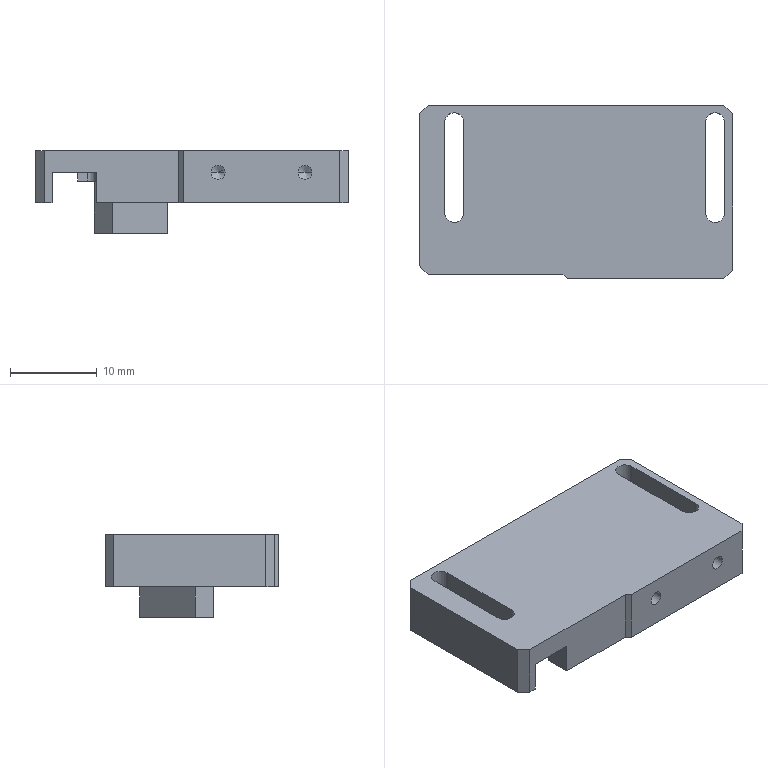NC program | NX | posted with a generic post | part box 36 x 20 x 9.5 mm
Lines 1 to 1629 of 4561:
N10 G17 G21 G94 G90
(FLOOR_WALL , TOOL : D10JING)
N12 T09 M6
N14 G54
N16 G17 G0 G90 X28. Y-11.997 S9500 M3
N18 G43 Z30. H9
N20 Z3.
N22 G94 G1 Z0. F1250.
N24 X25.
N26 X-25.
N28 Y-6.998
N30 X25.
N32 Y-1.999
N34 X-25.
N36 Y3.001
N38 X25.
N40 Y8.
N42 X-25.
N44 X-28.
N46 Z3.
N48 G0 Z30.
N50 M5
(ZLEVEL_PROFILE , TOOL : D10)
N52 T10 M6
N54 G54
N56 G17 G0 G90 X15.885 Y15.1 S9500 M3
N58 G43 Z30. H10
N60 Z1.5
N62 G94 G1 X17.554 Z1.413 F1000.
N64 X18.963 Y14.74 Z1.336
N66 X20.215 Y13.998 Z1.26
N68 X21.998 Y12.215 Z1.128
N70 X22.74 Y10.963 Z1.052
N72 X23.1 Y9.554 Z0.975
N74 Y-9.554 Z-0.026
N76 X22.74 Y-10.963 Z-0.102
N78 X21.998 Y-12.215 Z-0.178
N80 X20.215 Y-13.998 Z-0.311
N82 X18.963 Y-14.74 Z-0.387
N84 X17.554 Y-15.1 Z-0.463
N86 X17. Z-0.492
N88 X-17. F2500.
N90 G2 X-20.606 Y-13.606 R5.1
N92 G1 X-21.606 Y-12.606
N94 G2 X-23.1 Y-9. R5.1
N96 G1 Y8.5
N98 G2 X-21.606 Y12.106 R5.1
N100 G1 X-20.606 Y13.106
N102 G2 X-17. Y14.6 R5.1
N104 G1 X-3.202
N106 G2 X-1. Y15.1 R5.1
N108 G1 X17.
N110 G2 X20.606 Y13.606 R5.1
N112 G1 X21.606 Y12.606
N114 G2 X23.1 Y9. R5.1
N116 G1 Y-9.
N118 G2 X21.606 Y-12.606 R5.1
N120 G1 X20.606 Y-13.606
N122 G2 X17. Y-15.1 R5.1
N124 G1 X-11.193 Z-0.984
N126 X-17.
N128 G2 X-20.606 Y-13.606 R5.1
N130 G1 X-21.606 Y-12.606
N132 G2 X-23.1 Y-9. R5.1
N134 G1 Y8.5
N136 G2 X-21.606 Y12.106 R5.1
N138 G1 X-20.606 Y13.106
N140 G2 X-17. Y14.6 R5.1
N142 G1 X-3.202
N144 G2 X-1. Y15.1 R5.1
N146 G1 X17.
N148 G2 X20.606 Y13.606 R5.1
N150 G1 X21.606 Y12.606
N152 G2 X23.1 Y9. R5.1
N154 G1 Y-9.
N156 G2 X21.606 Y-12.606 R5.1
N158 G1 X20.606 Y-13.606
N160 G2 X17. Y-15.1 R5.1
N162 G1 X-11.193 Z-1.476
N164 X-17.
N166 G2 X-20.606 Y-13.606 R5.1
N168 G1 X-21.606 Y-12.606
N170 G2 X-23.1 Y-9. R5.1
N172 G1 Y8.5
N174 G2 X-21.606 Y12.106 R5.1
N176 G1 X-20.606 Y13.106
N178 G2 X-17. Y14.6 R5.1
N180 G1 X-3.202
N182 G2 X-1. Y15.1 R5.1
N184 G1 X17.
N186 G2 X20.606 Y13.606 R5.1
N188 G1 X21.606 Y12.606
N190 G2 X23.1 Y9. R5.1
N192 G1 Y-9.
N194 G2 X21.606 Y-12.606 R5.1
N196 G1 X20.606 Y-13.606
N198 G2 X17. Y-15.1 R5.1
N200 G1 X-11.193 Z-1.968
N202 X-17.
N204 G2 X-20.606 Y-13.606 R5.1
N206 G1 X-21.606 Y-12.606
N208 G2 X-23.1 Y-9. R5.1
N210 G1 Y8.5
N212 G2 X-21.606 Y12.106 R5.1
N214 G1 X-20.606 Y13.106
N216 G2 X-17. Y14.6 R5.1
N218 G1 X-3.202
N220 G2 X-1. Y15.1 R5.1
N222 G1 X17.
N224 G2 X20.606 Y13.606 R5.1
N226 G1 X21.606 Y12.606
N228 G2 X23.1 Y9. R5.1
N230 G1 Y-9.
N232 G2 X21.606 Y-12.606 R5.1
N234 G1 X20.606 Y-13.606
N236 G2 X17. Y-15.1 R5.1
N238 G1 X-11.193 Z-2.461
N240 X-17.
N242 G2 X-20.606 Y-13.606 R5.1
N244 G1 X-21.606 Y-12.606
N246 G2 X-23.1 Y-9. R5.1
N248 G1 Y8.5
N250 G2 X-21.606 Y12.106 R5.1
N252 G1 X-20.606 Y13.106
N254 G2 X-17. Y14.6 R5.1
N256 G1 X-3.202
N258 G2 X-1. Y15.1 R5.1
N260 G1 X17.
N262 G2 X20.606 Y13.606 R5.1
N264 G1 X21.606 Y12.606
N266 G2 X23.1 Y9. R5.1
N268 G1 Y-9.
N270 G2 X21.606 Y-12.606 R5.1
N272 G1 X20.606 Y-13.606
N274 G2 X17. Y-15.1 R5.1
N276 G1 X-11.193 Z-2.953
N278 X-17.
N280 G2 X-20.606 Y-13.606 R5.1
N282 G1 X-21.606 Y-12.606
N284 G2 X-23.1 Y-9. R5.1
N286 G1 Y8.5
N288 G2 X-21.606 Y12.106 R5.1
N290 G1 X-20.606 Y13.106
N292 G2 X-17. Y14.6 R5.1
N294 G1 X-3.202
N296 G2 X-1. Y15.1 R5.1
N298 G1 X17.
N300 G2 X20.606 Y13.606 R5.1
N302 G1 X21.606 Y12.606
N304 G2 X23.1 Y9. R5.1
N306 G1 Y-9.
N308 G2 X21.606 Y-12.606 R5.1
N310 G1 X20.606 Y-13.606
N312 G2 X17. Y-15.1 R5.1
N314 G1 X-11.193 Z-3.445
N316 X-17.
N318 G2 X-20.606 Y-13.606 R5.1
N320 G1 X-21.606 Y-12.606
N322 G2 X-23.1 Y-9. R5.1
N324 G1 Y8.5
N326 G2 X-21.606 Y12.106 R5.1
N328 G1 X-20.606 Y13.106
N330 G2 X-17. Y14.6 R5.1
N332 G1 X-3.202
N334 G2 X-1. Y15.1 R5.1
N336 G1 X17.
N338 G2 X20.606 Y13.606 R5.1
N340 G1 X21.606 Y12.606
N342 G2 X23.1 Y9. R5.1
N344 G1 Y-9.
N346 G2 X21.606 Y-12.606 R5.1
N348 G1 X20.606 Y-13.606
N350 G2 X17. Y-15.1 R5.1
N352 G1 X-11.193 Z-3.937
N354 X-17.
N356 G2 X-20.606 Y-13.606 R5.1
N358 G1 X-21.606 Y-12.606
N360 G2 X-23.1 Y-9. R5.1
N362 G1 Y8.5
N364 G2 X-21.606 Y12.106 R5.1
N366 G1 X-20.606 Y13.106
N368 G2 X-17. Y14.6 R5.1
N370 G1 X-3.202
N372 G2 X-1. Y15.1 R5.1
N374 G1 X17.
N376 G2 X20.606 Y13.606 R5.1
N378 G1 X21.606 Y12.606
N380 G2 X23.1 Y9. R5.1
N382 G1 Y-9.
N384 G2 X21.606 Y-12.606 R5.1
N386 G1 X20.606 Y-13.606
N388 G2 X17. Y-15.1 R5.1
N390 G1 X-11.193 Z-4.429
N392 X-17.
N394 G2 X-20.606 Y-13.606 R5.1
N396 G1 X-21.606 Y-12.606
N398 G2 X-23.1 Y-9. R5.1
N400 G1 Y8.5
N402 G2 X-21.606 Y12.106 R5.1
N404 G1 X-20.606 Y13.106
N406 G2 X-17. Y14.6 R5.1
N408 G1 X-3.202
N410 G2 X-1. Y15.1 R5.1
N412 G1 X17.
N414 G2 X20.606 Y13.606 R5.1
N416 G1 X21.606 Y12.606
N418 G2 X23.1 Y9. R5.1
N420 G1 Y-9.
N422 G2 X21.606 Y-12.606 R5.1
N424 G1 X20.606 Y-13.606
N426 G2 X17. Y-15.1 R5.1
N428 G1 X-11.193 Z-4.921
N430 X-17.
N432 G2 X-20.606 Y-13.606 R5.1
N434 G1 X-21.606 Y-12.606
N436 G2 X-23.1 Y-9. R5.1
N438 G1 Y8.5
N440 G2 X-21.606 Y12.106 R5.1
N442 G1 X-20.606 Y13.106
N444 G2 X-17. Y14.6 R5.1
N446 G1 X-3.202
N448 G2 X-1. Y15.1 R5.1
N450 G1 X17.
N452 G2 X20.606 Y13.606 R5.1
N454 G1 X21.606 Y12.606
N456 G2 X23.1 Y9. R5.1
N458 G1 Y-9.
N460 G2 X21.606 Y-12.606 R5.1
N462 G1 X20.606 Y-13.606
N464 G2 X17. Y-15.1 R5.1
N466 G1 X-11.193 Z-5.413
N468 X-17.
N470 G2 X-20.606 Y-13.606 R5.1
N472 G1 X-21.606 Y-12.606
N474 G2 X-23.1 Y-9. R5.1
N476 G1 Y8.5
N478 G2 X-21.606 Y12.106 R5.1
N480 G1 X-20.606 Y13.106
N482 G2 X-17. Y14.6 R5.1
N484 G1 X-3.202
N486 G2 X-1. Y15.1 R5.1
N488 G1 X17.
N490 G2 X20.606 Y13.606 R5.1
N492 G1 X21.606 Y12.606
N494 G2 X23.1 Y9. R5.1
N496 G1 Y-9.
N498 G2 X21.606 Y-12.606 R5.1
N500 G1 X20.606 Y-13.606
N502 G2 X17. Y-15.1 R5.1
N504 G1 X-11.193 Z-5.905
N506 X-17.
N508 G2 X-20.606 Y-13.606 R5.1
N510 G1 X-21.606 Y-12.606
N512 G2 X-23.1 Y-9. R5.1
N514 G1 Y8.5
N516 G2 X-21.606 Y12.106 R5.1
N518 G1 X-20.606 Y13.106
N520 G2 X-17. Y14.6 R5.1
N522 G1 X-3.202
N524 G2 X-1. Y15.1 R5.1
N526 G1 X17.
N528 G2 X20.606 Y13.606 R5.1
N530 G1 X21.606 Y12.606
N532 G2 X23.1 Y9. R5.1
N534 G1 Y-9.
N536 G2 X21.606 Y-12.606 R5.1
N538 G1 X20.606 Y-13.606
N540 G2 X17. Y-15.1 R5.1
N542 G1 X-11.193 Z-6.397
N544 X-17.
N546 G2 X-20.606 Y-13.606 R5.1
N548 G1 X-21.606 Y-12.606
N550 G2 X-23.1 Y-9. R5.1
N552 G1 Y8.5
N554 G2 X-21.606 Y12.106 R5.1
N556 G1 X-20.606 Y13.106
N558 G2 X-17. Y14.6 R5.1
N560 G1 X-3.202
N562 G2 X-1. Y15.1 R5.1
N564 G1 X17.
N566 G2 X20.606 Y13.606 R5.1
N568 G1 X21.606 Y12.606
N570 G2 X23.1 Y9. R5.1
N572 G1 Y-9.
N574 G2 X21.606 Y-12.606 R5.1
N576 G1 X20.606 Y-13.606
N578 G2 X17. Y-15.1 R5.1
N580 G1 X-11.193 Z-6.889
N582 X-17.
N584 G2 X-20.606 Y-13.606 R5.1
N586 G1 X-21.606 Y-12.606
N588 G2 X-23.1 Y-9. R5.1
N590 G1 Y8.5
N592 G2 X-21.606 Y12.106 R5.1
N594 G1 X-20.606 Y13.106
N596 G2 X-17. Y14.6 R5.1
N598 G1 X-3.202
N600 G2 X-1. Y15.1 R5.1
N602 G1 X17.
N604 G2 X20.606 Y13.606 R5.1
N606 G1 X21.606 Y12.606
N608 G2 X23.1 Y9. R5.1
N610 G1 Y-9.
N612 G2 X21.606 Y-12.606 R5.1
N614 G1 X20.606 Y-13.606
N616 G2 X17. Y-15.1 R5.1
N618 G1 X-11.193 Z-7.382
N620 X-17.
N622 G2 X-20.606 Y-13.606 R5.1
N624 G1 X-21.606 Y-12.606
N626 G2 X-23.1 Y-9. R5.1
N628 G1 Y8.5
N630 G2 X-21.606 Y12.106 R5.1
N632 G1 X-20.606 Y13.106
N634 G2 X-17. Y14.6 R5.1
N636 G1 X-3.202
N638 G2 X-1. Y15.1 R5.1
N640 G1 X17.
N642 G2 X20.606 Y13.606 R5.1
N644 G1 X21.606 Y12.606
N646 G2 X23.1 Y9. R5.1
N648 G1 Y-9.
N650 G2 X21.606 Y-12.606 R5.1
N652 G1 X20.606 Y-13.606
N654 G2 X17. Y-15.1 R5.1
N656 G1 X-11.193 Z-7.874
N658 X-17.
N660 G2 X-20.606 Y-13.606 R5.1
N662 G1 X-21.606 Y-12.606
N664 G2 X-23.1 Y-9. R5.1
N666 G1 Y8.5
N668 G2 X-21.606 Y12.106 R5.1
N670 G1 X-20.606 Y13.106
N672 G2 X-17. Y14.6 R5.1
N674 G1 X-3.202
N676 G2 X-1. Y15.1 R5.1
N678 G1 X17.
N680 G2 X20.606 Y13.606 R5.1
N682 G1 X21.606 Y12.606
N684 G2 X23.1 Y9. R5.1
N686 G1 Y-9.
N688 G2 X21.606 Y-12.606 R5.1
N690 G1 X20.606 Y-13.606
N692 G2 X17. Y-15.1 R5.1
N694 G1 X-11.193 Z-8.366
N696 X-17.
N698 G2 X-20.606 Y-13.606 R5.1
N700 G1 X-21.606 Y-12.606
N702 G2 X-23.1 Y-9. R5.1
N704 G1 Y8.5
N706 G2 X-21.606 Y12.106 R5.1
N708 G1 X-20.606 Y13.106
N710 G2 X-17. Y14.6 R5.1
N712 G1 X-3.202
N714 G2 X-1. Y15.1 R5.1
N716 G1 X17.
N718 G2 X20.606 Y13.606 R5.1
N720 G1 X21.606 Y12.606
N722 G2 X23.1 Y9. R5.1
N724 G1 Y-9.
N726 G2 X21.606 Y-12.606 R5.1
N728 G1 X20.606 Y-13.606
N730 G2 X17. Y-15.1 R5.1
N732 G1 X-11.193 Z-8.858
N734 X-17.
N736 G2 X-20.606 Y-13.606 R5.1
N738 G1 X-21.606 Y-12.606
N740 G2 X-23.1 Y-9. R5.1
N742 G1 Y8.5
N744 G2 X-21.606 Y12.106 R5.1
N746 G1 X-20.606 Y13.106
N748 G2 X-17. Y14.6 R5.1
N750 G1 X-3.202
N752 G2 X-1. Y15.1 R5.1
N754 G1 X17.
N756 G2 X20.606 Y13.606 R5.1
N758 G1 X21.606 Y12.606
N760 G2 X23.1 Y9. R5.1
N762 G1 Y-9.
N764 G2 X21.606 Y-12.606 R5.1
N766 G1 X20.606 Y-13.606
N768 G2 X17. Y-15.1 R5.1
N770 G1 X-11.193 Z-9.35
N772 X-17.
N774 G2 X-20.606 Y-13.606 R5.1
N776 G1 X-21.606 Y-12.606
N778 G2 X-23.1 Y-9. R5.1
N780 G1 Y8.5
N782 G2 X-21.606 Y12.106 R5.1
N784 G1 X-20.606 Y13.106
N786 G2 X-17. Y14.6 R5.1
N788 G1 X-3.202
N790 G2 X-1. Y15.1 R5.1
N792 G1 X17.
N794 G2 X20.606 Y13.606 R5.1
N796 G1 X21.606 Y12.606
N798 G2 X23.1 Y9. R5.1
N800 G1 Y-9.
N802 G2 X21.606 Y-12.606 R5.1
N804 G1 X20.606 Y-13.606
N806 G2 X17. Y-15.1 R5.1
N808 G1 X-11.193
N810 Z-7.85
N812 G0 Z30.
(CAVITY_MILL , TOOL : D10)
N814 X3.084 Y19.799
N816 Z1.014
N818 G1 Z-0.486 F1000.
N820 X7.126 Y12.799
N822 G3 X7.992 Y12.299 R1.
N824 G1 X19.531 F3000.
N826 X20.128 Y12.27
N828 X20.227 Y12.237
N830 X20.264 Y12.139
N832 X20.299 Y11.625
N834 Y-11.625
N836 X20.264 Y-12.139
N838 X20.227 Y-12.237
N840 X20.128 Y-12.27
N842 X19.531 Y-12.299
N844 X-3.356
N846 G2 X-6.443 Y-12.299 R6.5
N848 G1 X-19.531
N850 X-20.128 Y-12.27
N852 X-20.227 Y-12.237
N854 X-20.264 Y-12.139
N856 X-20.299 Y-11.625
N858 Y11.625
N860 X-20.264 Y12.139
N862 X-20.227 Y12.237
N864 X-20.128 Y12.27
N866 X-19.531 Y12.299
N868 X7.992
N870 Y5.299
N872 X13.299
N874 Y-5.299
N876 X3.561
N878 G3 X1.818 Y0.732 R6.5
N880 G1 X-2.749 Y5.299
N882 X-3.739 Y4.309
N884 X0.828 Y-0.258
N886 G2 X0.828 Y-7.47 R5.1
N888 G1 X-1.293 Y-9.592
N890 G2 X-8.506 Y-9.592 R5.1
N892 G1 X-14.87 Y-3.228
N894 G2 X-14.87 Y3.985 R5.1
N896 G1 X-12.748 Y6.106
N898 G2 X-5.536 Y6.106 R5.1
N900 G1 X-3.739 Y4.309
N902 X-2.749 Y5.299
N904 X7.992
N906 Y0.799
N908 X8.799
N910 Y-0.799
N912 X7.786
N914 G3 X7.184 Y0.799 R11.
N916 G1 X7.992
N918 G3 X8.858 Y1.299 R1.
N920 G1 Z1.014
N922 G0 Z30.
N924 X3.084 Y19.799
N926 Z0.529
N928 G1 Z-0.971 F1000.
N930 X7.126 Y12.799
N932 G3 X7.992 Y12.299 R1.
N934 G1 X19.531 F3000.
N936 X20.128 Y12.27
N938 X20.227 Y12.237
N940 X20.264 Y12.139
N942 X20.299 Y11.625
N944 Y-11.625
N946 X20.264 Y-12.139
N948 X20.227 Y-12.237
N950 X20.128 Y-12.27
N952 X19.531 Y-12.299
N954 X-3.356
N956 G2 X-6.443 Y-12.299 R6.5
N958 G1 X-19.531
N960 X-20.128 Y-12.27
N962 X-20.227 Y-12.237
N964 X-20.264 Y-12.139
N966 X-20.299 Y-11.625
N968 Y11.625
N970 X-20.264 Y12.139
N972 X-20.227 Y12.237
N974 X-20.128 Y12.27
N976 X-19.531 Y12.299
N978 X7.992
N980 Y5.299
N982 X13.299
N984 Y-5.299
N986 X3.561
N988 G3 X1.818 Y0.732 R6.5
N990 G1 X-2.749 Y5.299
N992 X-3.739 Y4.309
N994 X0.828 Y-0.258
N996 G2 X0.828 Y-7.47 R5.1
N998 G1 X-1.293 Y-9.592
N1000 G2 X-8.506 Y-9.592 R5.1
N1002 G1 X-14.87 Y-3.228
N1004 G2 X-14.87 Y3.985 R5.1
N1006 G1 X-12.748 Y6.106
N1008 G2 X-5.536 Y6.106 R5.1
N1010 G1 X-3.739 Y4.309
N1012 X-2.749 Y5.299
N1014 X7.992
N1016 Y0.799
N1018 X8.799
N1020 Y-0.799
N1022 X7.786
N1024 G3 X7.184 Y0.799 R11.
N1026 G1 X7.992
N1028 G3 X8.858 Y1.299 R1.
N1030 G1 Z0.529
N1032 G0 Z30.
N1034 X3.084 Y19.799
N1036 Z0.043
N1038 G1 Z-1.457 F1000.
N1040 X7.126 Y12.799
N1042 G3 X7.992 Y12.299 R1.
N1044 G1 X19.531 F3000.
N1046 X20.128 Y12.27
N1048 X20.228 Y12.237
N1050 X20.264 Y12.139
N1052 X20.299 Y11.625
N1054 Y-11.625
N1056 X20.264 Y-12.139
N1058 X20.228 Y-12.237
N1060 X20.128 Y-12.27
N1062 X19.531 Y-12.299
N1064 X-3.356
N1066 G2 X-6.443 Y-12.299 R6.5
N1068 G1 X-19.531
N1070 X-20.128 Y-12.27
N1072 X-20.228 Y-12.237
N1074 X-20.264 Y-12.139
N1076 X-20.299 Y-11.625
N1078 Y11.625
N1080 X-20.264 Y12.139
N1082 X-20.228 Y12.237
N1084 X-20.128 Y12.27
N1086 X-19.531 Y12.299
N1088 X7.992
N1090 Y5.299
N1092 X13.299
N1094 Y-5.299
N1096 X3.561
N1098 G3 X1.818 Y0.732 R6.5
N1100 G1 X-2.749 Y5.299
N1102 X-3.739 Y4.309
N1104 X0.828 Y-0.258
N1106 G2 X0.828 Y-7.47 R5.1
N1108 G1 X-1.293 Y-9.592
N1110 G2 X-8.506 Y-9.592 R5.1
N1112 G1 X-14.87 Y-3.228
N1114 G2 X-14.87 Y3.985 R5.1
N1116 G1 X-12.748 Y6.106
N1118 G2 X-5.536 Y6.106 R5.1
N1120 G1 X-3.739 Y4.309
N1122 X-2.749 Y5.299
N1124 X7.992
N1126 Y0.799
N1128 X8.799
N1130 Y-0.799
N1132 X7.786
N1134 G3 X7.184 Y0.799 R11.
N1136 G1 X7.992
N1138 G3 X8.858 Y1.299 R1.
N1140 G1 Z0.043
N1142 G0 X3.084 Y19.799 Z-0.443
N1144 G1 Z-1.943 F1000.
N1146 X7.126 Y12.799
N1148 G3 X7.992 Y12.299 R1.
N1150 G1 X19.531 F3000.
N1152 X20.128 Y12.27
N1154 X20.228 Y12.237
N1156 X20.264 Y12.139
N1158 X20.299 Y11.625
N1160 Y-11.625
N1162 X20.264 Y-12.139
N1164 X20.228 Y-12.237
N1166 X20.128 Y-12.27
N1168 X19.531 Y-12.299
N1170 X-3.356
N1172 G2 X-6.443 Y-12.299 R6.5
N1174 G1 X-19.531
N1176 X-20.128 Y-12.27
N1178 X-20.228 Y-12.237
N1180 X-20.264 Y-12.139
N1182 X-20.299 Y-11.625
N1184 Y11.625
N1186 X-20.264 Y12.139
N1188 X-20.228 Y12.237
N1190 X-20.128 Y12.27
N1192 X-19.531 Y12.299
N1194 X7.992
N1196 Y5.299
N1198 X13.299
N1200 Y-5.299
N1202 X3.561
N1204 G3 X1.818 Y0.732 R6.5
N1206 G1 X-2.749 Y5.299
N1208 X-3.739 Y4.31
N1210 X0.828 Y-0.258
N1212 G2 X0.828 Y-7.47 R5.1
N1214 G1 X-1.293 Y-9.592
N1216 G2 X-8.506 Y-9.592 R5.1
N1218 G1 X-14.87 Y-3.228
N1220 G2 X-14.87 Y3.985 R5.1
N1222 G1 X-12.748 Y6.106
N1224 G2 X-5.536 Y6.106 R5.1
N1226 G1 X-3.739 Y4.31
N1228 X-2.749 Y5.299
N1230 X7.992
N1232 Y0.799
N1234 X8.799
N1236 Y-0.799
N1238 X7.786
N1240 G3 X7.184 Y0.799 R11.
N1242 G1 X7.992
N1244 G3 X8.858 Y1.299 R1.
N1246 G1 Z-0.443
N1248 G0 X3.084 Y19.799 Z-0.929
N1250 G1 Z-2.429 F1000.
N1252 X7.126 Y12.799
N1254 G3 X7.992 Y12.299 R1.
N1256 G1 X19.531 F3000.
N1258 X20.129 Y12.27
N1260 X20.228 Y12.237
N1262 X20.264 Y12.139
N1264 X20.299 Y11.625
N1266 Y-11.625
N1268 X20.264 Y-12.139
N1270 X20.228 Y-12.237
N1272 X20.129 Y-12.27
N1274 X19.531 Y-12.299
N1276 X-3.357
N1278 G2 X-6.442 Y-12.299 R6.5
N1280 G1 X-19.531
N1282 X-20.129 Y-12.27
N1284 X-20.228 Y-12.237
N1286 X-20.264 Y-12.139
N1288 X-20.299 Y-11.625
N1290 Y11.625
N1292 X-20.264 Y12.139
N1294 X-20.228 Y12.237
N1296 X-20.129 Y12.27
N1298 X-19.531 Y12.299
N1300 X7.992
N1302 Y5.299
N1304 X13.299
N1306 Y-5.299
N1308 X3.561
N1310 G3 X1.818 Y0.732 R6.5
N1312 G1 X-2.749 Y5.299
N1314 X-3.739 Y4.31
N1316 X0.828 Y-0.258
N1318 G2 X0.828 Y-7.47 R5.1
N1320 G1 X-1.293 Y-9.592
N1322 G2 X-8.506 Y-9.592 R5.1
N1324 G1 X-14.87 Y-3.228
N1326 G2 X-14.87 Y3.985 R5.1
N1328 G1 X-12.748 Y6.106
N1330 G2 X-5.536 Y6.106 R5.1
N1332 G1 X-3.739 Y4.31
N1334 X-2.749 Y5.299
N1336 X7.992
N1338 Y0.799
N1340 X8.799
N1342 Y-0.799
N1344 X7.786
N1346 G3 X7.184 Y0.799 R11.
N1348 G1 X7.992
N1350 G3 X8.858 Y1.299 R1.
N1352 G1 Z-0.929
N1354 G0 X3.084 Y19.8 Z-1.414
N1356 G1 Z-2.914 F1000.
N1358 X7.126 Y12.8
N1360 G3 X7.992 Y12.3 R1.
N1362 G1 X19.531 F3000.
N1364 X20.129 Y12.27
N1366 X20.228 Y12.237
N1368 X20.264 Y12.139
N1370 X20.3 Y11.625
N1372 Y-11.625
N1374 X20.264 Y-12.139
N1376 X20.228 Y-12.237
N1378 X20.129 Y-12.27
N1380 X19.531 Y-12.3
N1382 X-3.357
N1384 G2 X-6.442 Y-12.3 R6.5
N1386 G1 X-19.531
N1388 X-20.129 Y-12.27
N1390 X-20.228 Y-12.237
N1392 X-20.264 Y-12.139
N1394 X-20.3 Y-11.625
N1396 Y11.625
N1398 X-20.264 Y12.139
N1400 X-20.228 Y12.237
N1402 X-20.129 Y12.27
N1404 X-19.531 Y12.3
N1406 X7.992
N1408 Y5.3
N1410 X13.3
N1412 Y-5.3
N1414 X3.561
N1416 G3 X1.818 Y0.732 R6.5
N1418 G1 X-2.749 Y5.3
N1420 X-3.739 Y4.31
N1422 X0.828 Y-0.258
N1424 G2 X0.828 Y-7.47 R5.1
N1426 G1 X-1.293 Y-9.592
N1428 G2 X-8.506 Y-9.592 R5.1
N1430 G1 X-14.87 Y-3.228
N1432 G2 X-14.87 Y3.985 R5.1
N1434 G1 X-12.748 Y6.106
N1436 G2 X-5.536 Y6.106 R5.1
N1438 G1 X-3.739 Y4.31
N1440 X-2.749 Y5.3
N1442 X7.992
N1444 Y0.8
N1446 X8.8
N1448 Y-0.8
N1450 X7.786
N1452 G3 X7.184 Y0.8 R11.
N1454 G1 X7.992
N1456 G3 X8.858 Y1.3 R1.
N1458 G1 Z-1.414
N1460 G0 X3.084 Y19.8 Z-1.9
N1462 G1 Z-3.4 F1000.
N1464 X7.126 Y12.8
N1466 G3 X7.992 Y12.3 R1.
N1468 G1 X19.531 F3000.
N1470 X20.129 Y12.27
N1472 X20.228 Y12.237
N1474 X20.264 Y12.139
N1476 X20.3 Y11.625
N1478 Y-11.625
N1480 X20.264 Y-12.139
N1482 X20.228 Y-12.237
N1484 X20.129 Y-12.27
N1486 X19.531 Y-12.3
N1488 X-3.357
N1490 G2 X-6.442 Y-12.3 R6.5
N1492 G1 X-19.531
N1494 X-20.129 Y-12.27
N1496 X-20.228 Y-12.237
N1498 X-20.264 Y-12.139
N1500 X-20.3 Y-11.625
N1502 Y11.625
N1504 X-20.264 Y12.139
N1506 X-20.228 Y12.237
N1508 X-20.129 Y12.27
N1510 X-19.531 Y12.3
N1512 X7.992
N1514 Y5.3
N1516 X13.3
N1518 Y-5.3
N1520 X3.561
N1522 G3 X1.818 Y0.732 R6.5
N1524 G1 X-2.749 Y5.3
N1526 X-3.739 Y4.31
N1528 X0.828 Y-0.258
N1530 G2 X0.828 Y-7.47 R5.1
N1532 G1 X-1.293 Y-9.592
N1534 G2 X-8.506 Y-9.592 R5.1
N1536 G1 X-14.87 Y-3.228
N1538 G2 X-14.87 Y3.985 R5.1
N1540 G1 X-12.748 Y6.106
N1542 G2 X-5.536 Y6.106 R5.1
N1544 G1 X-3.739 Y4.31
N1546 X-2.749 Y5.3
N1548 X7.992
N1550 Y0.8
N1552 X8.8
N1554 Y-0.8
N1556 X7.786
N1558 G3 X7.184 Y0.8 R11.
N1560 G1 X7.992
N1562 G3 X8.858 Y1.3 R1.
N1564 G1 Z-1.9
N1566 G0 X27.8 Y-5.101 Z-2.4
N1568 G1 Z-3.9 F1000.
N1570 X23.5 Y-2.619
N1572 G2 X23. Y-1.752 R1.
N1574 G1 Y5.495 F3000.
N1576 G2 X19. Y1.499 R5.1
N1578 G1 Y-10.
N1580 G2 X14.905 Y-15. R5.1
N1582 G1 X17.
N1584 G3 X20.536 Y-13.536 R5.
N1586 G1 X21.536 Y-12.536
N1588 G3 X23. Y-9. R5.
N1590 G1 Y-1.752
N1592 G2 X23.5 Y-0.886 R1.
N1594 G1 X27.8 Y1.596
N1596 Z-2.4
N1598 G0 Y-5.101 Z-2.9
N1600 G1 Z-4.4 F1000.
N1602 X23.5 Y-2.619
N1604 G2 X23. Y-1.752 R1.
N1606 G1 Y5.495 F3000.
N1608 G2 X19. Y1.499 R5.1
N1610 G1 Y-10.
N1612 G2 X14.905 Y-15. R5.1
N1614 G1 X17.
N1616 G3 X20.536 Y-13.536 R5.
N1618 G1 X21.536 Y-12.536
N1620 G3 X23. Y-9. R5.
N1622 G1 Y-1.752
N1624 G2 X23.5 Y-0.886 R1.
N1626 G1 X27.8 Y1.596
N1628 Z-2.9
N1630 G0 Y-5.101 Z-3.4
N1632 G1 Z-4.9 F1000.
N1634 X23.5 Y-2.619
N1636 G2 X23. Y-1.752 R1.
N1638 G1 Y5.495 F3000.
N1640 G2 X19. Y1.499 R5.1
N1642 G1 Y-10.
N1644 G2 X14.905 Y-15. R5.1
N1646 G1 X17.
N1648 G3 X20.536 Y-13.536 R5.
N1650 G1 X21.536 Y-12.536
N1652 G3 X23. Y-9. R5.
N1654 G1 Y-1.752
N1656 G2 X23.5 Y-0.886 R1.
N1658 G1 X27.8 Y1.596
N1660 Z-3.4
N1662 G0 Y-5.101 Z-3.9
N1664 G1 Z-5.4 F1000.
N1666 X23.5 Y-2.619
N1668 G2 X23. Y-1.752 R1.
N1670 G1 Y5.495 F3000.
N1672 G2 X19. Y1.499 R5.1
N1674 G1 Y-10.
N1676 G2 X14.905 Y-15. R5.1
N1678 G1 X17.
N1680 G3 X20.536 Y-13.536 R5.
N1682 G1 X21.536 Y-12.536
N1684 G3 X23. Y-9. R5.
N1686 G1 Y-1.752
N1688 G2 X23.5 Y-0.886 R1.
N1690 G1 X27.8 Y1.596
N1692 Z-3.9
N1694 G0 Y-5.101 Z-4.4
N1696 G1 Z-5.9 F1000.
N1698 X23.5 Y-2.619
N1700 G2 X23. Y-1.752 R1.
N1702 G1 Y5.495 F3000.
N1704 G2 X19. Y1.499 R5.1
N1706 G1 Y-10.
N1708 G2 X14.905 Y-15. R5.1
N1710 G1 X17.
N1712 G3 X20.536 Y-13.536 R5.
N1714 G1 X21.536 Y-12.536
N1716 G3 X23. Y-9. R5.
N1718 G1 Y-1.752
N1720 G2 X23.5 Y-0.886 R1.
N1722 G1 X27.8 Y1.596
N1724 Z-4.4
N1726 G0 Y-5.101 Z-4.9
N1728 G1 Z-6.4 F1000.
N1730 X23.5 Y-2.619
N1732 G2 X23. Y-1.752 R1.
N1734 G1 Y5.495 F3000.
N1736 G2 X19. Y1.499 R5.1
N1738 G1 Y-10.
N1740 G2 X14.905 Y-15. R5.1
N1742 G1 X17.
N1744 G3 X20.536 Y-13.536 R5.
N1746 G1 X21.536 Y-12.536
N1748 G3 X23. Y-9. R5.
N1750 G1 Y-1.752
N1752 G2 X23.5 Y-0.886 R1.
N1754 G1 X27.8 Y1.596
N1756 Z-4.9
N1758 G0 Y-5.101 Z-5.4
N1760 G1 Z-6.9 F1000.
N1762 X23.5 Y-2.619
N1764 G2 X23. Y-1.752 R1.
N1766 G1 Y5.495 F3000.
N1768 G2 X19. Y1.499 R5.1
N1770 G1 Y-10.
N1772 G2 X14.905 Y-15. R5.1
N1774 G1 X17.
N1776 G3 X20.536 Y-13.536 R5.
N1778 G1 X21.536 Y-12.536
N1780 G3 X23. Y-9. R5.
N1782 G1 Y-1.752
N1784 G2 X23.5 Y-0.886 R1.
N1786 G1 X27.8 Y1.596
N1788 Z-5.4
N1790 G0 Z30.
N1792 X-4.176 Y-19.8
N1794 Z-2.4
N1796 G1 Z-3.9 F1000.
N1798 X-0.134 Y-12.8
N1800 G2 X0.732 Y-12.3 R1.
N1802 G1 X4.82 F3000.
N1804 G3 X6.747 Y-15. R6.5
N1806 G1 X9.895
N1808 G2 X5.8 Y-10. R5.1
N1810 G1 Y0.844
N1812 G2 X5.83 Y1.4 R5.1
N1814 G1 X-0.83
N1816 X0.828 Y-0.258
N1818 G2 X0.828 Y-7.47 R5.1
N1820 G1 X-1.293 Y-9.592
N1822 G2 X-8.506 Y-9.592 R5.1
N1824 G1 X-11. Y-7.097
N1826 Y-10.
N1828 G2 X-15.095 Y-15. R5.1
N1830 G1 X-11.947
N1832 G3 X-10.02 Y-12.3 R6.5
N1834 G1 X-6.442
N1836 G3 X-3.357 Y-12.3 R6.5
N1838 G1 X0.732
N1840 G2 X1.598 Y-12.8 R1.
N1842 G1 X5.639 Y-19.8
N1844 Z-2.4
N1846 G0 X-4.176 Z-2.9
N1848 G1 Z-4.4 F1000.
N1850 X-0.134 Y-12.8
N1852 G2 X0.732 Y-12.3 R1.
N1854 G1 X4.82 F3000.
N1856 G3 X6.747 Y-15. R6.5
N1858 G1 X9.895
N1860 G2 X5.8 Y-10. R5.1
N1862 G1 Y0.844
N1864 G2 X5.83 Y1.4 R5.1
N1866 G1 X-0.83
N1868 X0.828 Y-0.258
N1870 G2 X0.828 Y-7.47 R5.1
N1872 G1 X-1.293 Y-9.592
N1874 G2 X-8.506 Y-9.592 R5.1
N1876 G1 X-11. Y-7.097
N1878 Y-9.077
N1880 Y-10.
N1882 G2 X-15.095 Y-15. R5.1
N1884 G1 X-11.947
N1886 G3 X-10.02 Y-12.3 R6.5
N1888 G1 X-6.442
N1890 G3 X-3.357 Y-12.3 R6.5
N1892 G1 X0.732
N1894 G2 X1.598 Y-12.8 R1.
N1896 G1 X5.639 Y-19.8
N1898 Z-2.9
N1900 G0 X-4.176 Z-3.4
N1902 G1 Z-4.9 F1000.
N1904 X-0.134 Y-12.8
N1906 G2 X0.732 Y-12.3 R1.
N1908 G1 X4.82 F3000.
N1910 G3 X6.747 Y-15. R6.5
N1912 G1 X9.895
N1914 G2 X5.8 Y-10. R5.1
N1916 G1 Y0.844
N1918 G2 X5.83 Y1.4 R5.1
N1920 G1 X-0.83
N1922 X0.828 Y-0.258
N1924 G2 X0.828 Y-7.47 R5.1
N1926 G1 X-1.293 Y-9.592
N1928 G2 X-8.506 Y-9.592 R5.1
N1930 G1 X-11. Y-7.097
N1932 Y-10.
N1934 G2 X-15.095 Y-15. R5.1
N1936 G1 X-11.947
N1938 G3 X-10.02 Y-12.3 R6.5
N1940 G1 X-6.442
N1942 G3 X-3.357 Y-12.3 R6.5
N1944 G1 X0.732
N1946 G2 X1.598 Y-12.8 R1.
N1948 G1 X5.639 Y-19.8
N1950 Z-3.4
N1952 G0 X-4.176 Z-3.9
N1954 G1 Z-5.4 F1000.
N1956 X-0.135 Y-12.8
N1958 G2 X0.732 Y-12.3 R1.
N1960 G1 X4.82 F3000.
N1962 G3 X6.747 Y-15. R6.5
N1964 G1 X9.895
N1966 G2 X5.8 Y-10. R5.1
N1968 G1 Y0.844
N1970 G2 X5.83 Y1.4 R5.1
N1972 G1 X-0.83
N1974 X0.828 Y-0.258
N1976 G2 X0.828 Y-7.47 R5.1
N1978 G1 X-1.293 Y-9.592
N1980 G2 X-8.506 Y-9.592 R5.1
N1982 G1 X-11. Y-7.097
N1984 Y-10.
N1986 G2 X-15.095 Y-15. R5.1
N1988 G1 X-11.947
N1990 G3 X-10.02 Y-12.3 R6.5
N1992 G1 X-6.442
N1994 G3 X-3.357 Y-12.3 R6.5
N1996 G1 X0.732
N1998 G2 X1.598 Y-12.8 R1.
N2000 G1 X5.639 Y-19.8
N2002 Z-3.9
N2004 G0 X-4.176 Z-4.4
N2006 G1 Z-5.9 F1000.
N2008 X-0.135 Y-12.8
N2010 G2 X0.731 Y-12.3 R1.
N2012 G1 X4.82 F3000.
N2014 G3 X6.747 Y-15. R6.5
N2016 G1 X9.895
N2018 G2 X5.8 Y-10. R5.1
N2020 G1 Y0.844
N2022 G2 X5.83 Y1.4 R5.1
N2024 G1 X-0.83
N2026 X0.57 Y0.
N2028 X0.828 Y-0.258
N2030 G2 X0.828 Y-7.47 R5.1
N2032 G1 X-1.293 Y-9.592
N2034 G2 X-8.506 Y-9.592 R5.1
N2036 G1 X-11. Y-7.097
N2038 Y-9.077
N2040 Y-10.
N2042 G2 X-15.095 Y-15. R5.1
N2044 G1 X-11.947
N2046 G3 X-10.02 Y-12.3 R6.5
N2048 G1 X-6.441
N2050 G3 X-3.358 Y-12.3 R6.5
N2052 G1 X0.731
N2054 G2 X1.597 Y-12.8 R1.
N2056 G1 X5.639 Y-19.8
N2058 Z-4.4
N2060 G0 X-2.642 Z-4.9
N2062 G1 Z-6.4 F1000.
N2064 X-0.16 Y-15.5
N2066 G2 X0.706 Y-15. R1.
N2068 G1 X0.692 Y-12.983
N2070 X0.706 Y-12.734
N2072 G2 X-2.606 Y-11.248 R5.1 F3000.
N2074 G1 X-3.098 Y-10.757
N2076 G2 X-8.506 Y-9.592 R5.1
N2078 G1 X-11. Y-7.097
N2080 Y-10.
N2082 G2 X-15.095 Y-15. R5.1
N2084 G1 X9.895
N2086 G2 X5.8 Y-10.055 R5.1
N2088 G1 X4.606 Y-11.248
N2090 G2 X0.706 Y-12.734 R5.1
N2092 G3 X-0.187 Y-13.183 R1.
N2094 G1 Y-19.8
N2096 Z-4.9
N2098 G0 X-2.642 Z-5.4
N2100 G1 Z-6.9 F1000.
N2102 X-0.16 Y-15.5
N2104 G2 X0.706 Y-15. R1.
N2106 G1 X0.692 Y-12.983
N2108 X0.706 Y-12.734
N2110 G2 X-2.606 Y-11.248 R5.1 F3000.
N2112 G1 X-3.098 Y-10.757
N2114 G2 X-8.506 Y-9.592 R5.1
N2116 G1 X-11. Y-7.097
N2118 Y-10.
N2120 G2 X-15.095 Y-15. R5.1
N2122 G1 X9.895
N2124 G2 X5.8 Y-10.057 R5.1
N2126 G1 X4.606 Y-11.248
N2128 G2 X0.706 Y-12.734 R5.1
N2130 G3 X-0.187 Y-13.183 R1.
N2132 G1 Y-19.8
N2134 Z-5.4
N2136 G0 Z30.
N2138 X-10.086 Y19.5
N2140 Z-2.4
N2142 G1 Z-3.9 F1000.
N2144 X-12.684 Y15.
N2146 G2 X-13.55 Y14.5 R1.
N2148 G1 X-15.095 F3000.
N2150 G2 X-13.55 Y13.917 R5.1
N2152 X-12.005 Y14.5 R5.1
N2154 G1 X-13.55
N2156 G2 X-14.416 Y15. R1.
N2158 G1 X-17.014 Y19.5
N2160 Z-2.4
N2162 G0 X-10.086 Z-2.9
N2164 G1 Z-4.4 F1000.
N2166 X-12.684 Y15.
N2168 G2 X-13.55 Y14.5 R1.
N2170 G1 X-15.095 F3000.
N2172 G2 X-13.55 Y13.917 R5.1
N2174 X-12.005 Y14.5 R5.1
N2176 G1 X-13.55
N2178 G2 X-14.416 Y15. R1.
N2180 G1 X-17.014 Y19.5
N2182 Z-2.9
N2184 G0 X-10.086 Z-3.4
N2186 G1 Z-4.9 F1000.
N2188 X-12.684 Y15.
N2190 G2 X-13.55 Y14.5 R1.
N2192 G1 X-15.095 F3000.
N2194 G2 X-13.55 Y13.917 R5.1
N2196 X-12.005 Y14.5 R5.1
N2198 G1 X-13.55
N2200 G2 X-14.416 Y15. R1.
N2202 G1 X-17.014 Y19.5
N2204 Z-3.4
N2206 G0 X-10.086 Z-3.9
N2208 G1 Z-5.4 F1000.
N2210 X-12.684 Y15.
N2212 G2 X-13.55 Y14.5 R1.
N2214 G1 X-15.095 F3000.
N2216 G2 X-13.55 Y13.917 R5.1
N2218 X-12.005 Y14.5 R5.1
N2220 G1 X-13.55
N2222 G2 X-14.416 Y15. R1.
N2224 G1 X-17.014 Y19.5
N2226 Z-3.9
N2228 G0 X-10.086 Z-4.4
N2230 G1 Z-5.9 F1000.
N2232 X-12.684 Y15.
N2234 G2 X-13.55 Y14.5 R1.
N2236 G1 X-15.095 F3000.
N2238 G2 X-13.55 Y13.917 R5.1
N2240 X-12.005 Y14.5 R5.1
N2242 G1 X-13.55
N2244 G2 X-14.416 Y15. R1.
N2246 G1 X-17.014 Y19.5
N2248 Z-4.4
N2250 G0 X-10.086 Z-4.9
N2252 G1 Z-6.4 F1000.
N2254 X-12.684 Y15.
N2256 G2 X-13.55 Y14.5 R1.
N2258 G1 X-15.095 F3000.
N2260 G2 X-13.55 Y13.917 R5.1
N2262 X-12.005 Y14.5 R5.1
N2264 G1 X-13.55
N2266 G2 X-14.416 Y15. R1.
N2268 G1 X-17.014 Y19.5
N2270 Z-4.9
N2272 G0 X-10.086 Z-5.4
N2274 G1 Z-6.9 F1000.
N2276 X-12.684 Y15.
N2278 G2 X-13.55 Y14.5 R1.
N2280 G1 X-15.095 F3000.
N2282 G2 X-13.55 Y13.917 R5.1
N2284 X-12.005 Y14.5 R5.1
N2286 G1 X-13.55
N2288 G2 X-14.416 Y15. R1.
N2290 G1 X-17.014 Y19.5
N2292 Z-5.4
N2294 G0 Z30.
N2296 M5
(CAVITY_MILL_COPY , TOOL : D6)
N2298 T06 M6
N2300 G54
N2302 G17 G0 G90 X-9.711 Y-8.103 S9509 M3
N2304 G43 Z30. H6
N2306 Z-2.4
N2308 G94 G1 Z-3.9 F1000.
N2310 X-9.322 Y-6.654
N2312 G3 X-9.581 Y-5.688 R1.
N2314 G1 X-13. Y-2.269 F1500.
N2316 Y-7.104
N2318 G3 X-12.5 Y-7.97 R1.
N2320 G1 X-11.2 Y-8.72
N2322 Z-2.4
N2324 G0 X-9.711 Y-8.103 Z-2.9
N2326 G1 Z-4.4 F1000.
N2328 X-9.322 Y-6.654
N2330 G3 X-9.581 Y-5.688 R1.
N2332 G1 X-13. Y-2.269 F1500.
N2334 Y-7.104
N2336 G3 X-12.5 Y-7.97 R1.
N2338 G1 X-11.2 Y-8.72
N2340 Z-2.9
N2342 G0 X-9.711 Y-8.103 Z-3.4
N2344 G1 Z-4.9 F1000.
N2346 X-9.322 Y-6.654
N2348 G3 X-9.581 Y-5.688 R1.
N2350 G1 X-13. Y-2.269 F1500.
N2352 Y-7.104
N2354 G3 X-12.5 Y-7.97 R1.
N2356 G1 X-11.2 Y-8.72
N2358 Z-3.4
N2360 G0 X-9.711 Y-8.103 Z-3.9
N2362 G1 Z-5.4 F1000.
N2364 X-9.322 Y-6.654
N2366 G3 X-9.581 Y-5.688 R1.
N2368 G1 X-13. Y-2.269 F1500.
N2370 Y-7.104
N2372 G3 X-12.5 Y-7.97 R1.
N2374 G1 X-11.2 Y-8.72
N2376 Z-3.9
N2378 G0 X-9.711 Y-8.103 Z-4.4
N2380 G1 Z-5.9 F1000.
N2382 X-9.322 Y-6.654
N2384 G3 X-9.581 Y-5.688 R1.
N2386 G1 X-13. Y-2.269 F1500.
N2388 Y-7.104
N2390 G3 X-12.5 Y-7.97 R1.
N2392 G1 X-11.2 Y-8.72
N2394 Z-4.4
N2396 G0 X-9.711 Y-8.103 Z-4.9
N2398 G1 Z-6.4 F1000.
N2400 X-9.322 Y-6.654
N2402 G3 X-9.581 Y-5.688 R1.
N2404 G1 X-13. Y-2.269 F1500.
N2406 Y-7.104
N2408 G3 X-12.5 Y-7.97 R1.
N2410 G1 X-11.2 Y-8.72
N2412 Z-4.9
N2414 G0 X-9.711 Y-8.103 Z-5.4
N2416 G1 Z-6.9 F1000.
N2418 X-9.322 Y-6.654
N2420 G3 X-9.581 Y-5.688 R1.
N2422 G1 X-13. Y-2.269 F1500.
N2424 Y-7.104
N2426 G3 X-12.5 Y-7.97 R1.
N2428 G1 X-11.2 Y-8.72
N2430 Z-5.4
N2432 G0 Z30.
N2434 X-15.229 Y14.322
N2436 Z-2.4
N2438 G1 Z-3.9 F1000.
N2440 X-15.183 Y13.087
N2442 G3 X-14.651 Y12.241 R1.
N2444 G2 X-13.608 Y11.343 R3.1 F1500.
N2446 G1 X-13.52 Y11.305
N2448 G2 X-12.449 Y12.241 R3.1
N2450 G3 X-11.917 Y13.087 R1.
N2452 G1 X-11.871 Y14.322
N2454 Z-2.4
N2456 G0 X-15.229 Z-2.9
N2458 G1 Z-4.4 F1000.
N2460 X-15.183 Y13.087
N2462 G3 X-14.651 Y12.241 R1.
N2464 G2 X-13.608 Y11.343 R3.1 F1500.
N2466 G1 X-13.52 Y11.305
N2468 G2 X-12.449 Y12.241 R3.1
N2470 G3 X-11.917 Y13.087 R1.
N2472 G1 X-11.871 Y14.322
N2474 Z-2.9
N2476 G0 X-15.229 Z-3.4
N2478 G1 Z-4.9 F1000.
N2480 X-15.183 Y13.087
N2482 G3 X-14.651 Y12.241 R1.
N2484 G2 X-13.599 Y11.332 R3.1 F1500.
N2486 G1 X-13.52 Y11.305
N2488 G2 X-12.449 Y12.241 R3.1
N2490 G3 X-11.917 Y13.087 R1.
N2492 G1 X-11.871 Y14.322
N2494 Z-3.4
N2496 G0 X-15.229 Z-3.9
N2498 G1 Z-5.4 F1000.
N2500 X-15.183 Y13.087
N2502 G3 X-14.651 Y12.241 R1.
N2504 G2 X-13.599 Y11.332 R3.1 F1500.
N2506 G1 X-13.515 Y11.313
N2508 G2 X-12.449 Y12.241 R3.1
N2510 G3 X-11.917 Y13.087 R1.
N2512 G1 X-11.871 Y14.322
N2514 Z-3.9
N2516 G0 X-15.229 Z-4.4
N2518 G1 Z-5.9 F1000.
N2520 X-15.183 Y13.087
N2522 G3 X-14.651 Y12.241 R1.
N2524 G2 X-13.599 Y11.332 R3.1 F1500.
N2526 G1 X-13.515 Y11.313
N2528 G2 X-12.449 Y12.241 R3.1
N2530 G3 X-11.917 Y13.087 R1.
N2532 G1 X-11.871 Y14.322
N2534 Z-4.4
N2536 G0 X-15.229 Z-4.9
N2538 G1 Z-6.4 F1000.
N2540 X-15.183 Y13.087
N2542 G3 X-14.651 Y12.241 R1.
N2544 G2 X-13.599 Y11.332 R3.1 F1500.
N2546 G1 X-13.515 Y11.313
N2548 G2 X-12.449 Y12.241 R3.1
N2550 G3 X-11.917 Y13.087 R1.
N2552 G1 X-11.871 Y14.322
N2554 Z-4.9
N2556 G0 X-15.229 Z-5.4
N2558 G1 Z-6.9 F1000.
N2560 X-15.183 Y13.087
N2562 G3 X-14.651 Y12.241 R1.
N2564 G2 X-13.599 Y11.332 R3.1 F1500.
N2566 G1 X-13.515 Y11.313
N2568 G2 X-12.449 Y12.241 R3.1
N2570 G3 X-11.917 Y13.087 R1.
N2572 G1 X-11.871 Y14.322
N2574 Z-5.4
N2576 G0 Z30.
N2578 X-4.822 Y14.4
N2580 Z-2.4
N2582 G1 Z-3.9 F1000.
N2584 X-4.072 Y13.1
N2586 G3 X-3.206 Y12.6 R1.
N2588 G1 X-2.688 F1500.
N2590 G2 X-2.236 Y12.843 R3.1
N2592 G3 X-1.641 Y13.647 R1.
N2594 G1 X-1.501 Y14.874
N2596 Z-2.4
N2598 G0 X-4.825 Y14.4 Z-2.9
N2600 G1 Z-4.4 F1000.
N2602 X-4.075 Y13.1
N2604 G3 X-3.209 Y12.6 R1.
N2606 G1 X-2.688 F1500.
N2608 G2 X-2.234 Y12.844 R3.1
N2610 G3 X-1.638 Y13.647 R1.
N2612 G1 X-1.497 Y14.875
N2614 Z-2.9
N2616 G0 X-4.825 Y14.4 Z-3.4
N2618 G1 Z-4.9 F1000.
N2620 X-4.075 Y13.1
N2622 G3 X-3.209 Y12.6 R1.
N2624 G1 X-2.688 F1500.
N2626 G2 X-2.234 Y12.844 R3.1
N2628 G3 X-1.638 Y13.647 R1.
N2630 G1 X-1.497 Y14.875
N2632 Z-3.4
N2634 G0 X-4.825 Y14.4 Z-3.9
N2636 G1 Z-5.4 F1000.
N2638 X-4.075 Y13.1
N2640 G3 X-3.209 Y12.6 R1.
N2642 G1 X-2.688 F1500.
N2644 G2 X-2.234 Y12.844 R3.1
N2646 G3 X-1.638 Y13.647 R1.
N2648 G1 X-1.497 Y14.875
N2650 Z-3.9
N2652 G0 X-4.825 Y14.4 Z-4.4
N2654 G1 Z-5.9 F1000.
N2656 X-4.075 Y13.1
N2658 G3 X-3.209 Y12.6 R1.
N2660 G1 X-2.688 F1500.
N2662 G2 X-2.234 Y12.844 R3.1
N2664 G3 X-1.638 Y13.647 R1.
N2666 G1 X-1.497 Y14.875
N2668 Z-4.4
N2670 G0 X-4.825 Y14.4 Z-4.9
N2672 G1 Z-6.4 F1000.
N2674 X-4.075 Y13.1
N2676 G3 X-3.209 Y12.6 R1.
N2678 G1 X-2.688 F1500.
N2680 G2 X-2.234 Y12.844 R3.1
N2682 G3 X-1.638 Y13.647 R1.
N2684 G1 X-1.497 Y14.875
N2686 Z-4.9
N2688 G0 X-4.825 Y14.4 Z-5.4
N2690 G1 Z-6.9 F1000.
N2692 X-4.075 Y13.1
N2694 G3 X-3.209 Y12.6 R1.
N2696 G1 X-2.688 F1500.
N2698 G2 X-2.234 Y12.844 R3.1
N2700 G3 X-1.638 Y13.647 R1.
N2702 G1 X-1.497 Y14.875
N2704 Z-5.4
N2706 G0 X-4.825 Y14.4 Z-5.833
N2708 G1 Z-7.333 F1000.
N2710 X-4.075 Y13.1
N2712 G3 X-3.209 Y12.6 R1.
N2714 G1 X-2.688 F1500.
N2716 G2 X-2.234 Y12.844 R3.1
N2718 G3 X-1.638 Y13.647 R1.
N2720 G1 X-1.497 Y14.875
N2722 Z-5.833
N2724 G0 X-4.825 Y14.4 Z-6.267
N2726 G1 Z-7.767 F1000.
N2728 X-4.075 Y13.1
N2730 G3 X-3.209 Y12.6 R1.
N2732 G1 X-2.688 F1500.
N2734 G2 X-2.234 Y12.844 R3.1
N2736 G3 X-1.638 Y13.647 R1.
N2738 G1 X-1.497 Y14.875
N2740 Z-6.267
N2742 G0 X-4.825 Y14.4 Z-6.7
N2744 G1 Z-8.2 F1000.
N2746 X-4.075 Y13.1
N2748 G3 X-3.209 Y12.6 R1.
N2750 G1 X-2.688 F1500.
N2752 G2 X-2.234 Y12.844 R3.1
N2754 G3 X-1.638 Y13.647 R1.
N2756 G1 X-1.497 Y14.875
N2758 Z-6.7
N2760 G0 X-4.825 Y14.4 Z-7.133
N2762 G1 Z-8.633 F1000.
N2764 X-4.075 Y13.1
N2766 G3 X-3.209 Y12.6 R1.
N2768 G1 X-2.688 F1500.
N2770 G2 X-2.234 Y12.844 R3.1
N2772 G3 X-1.638 Y13.647 R1.
N2774 G1 X-1.497 Y14.875
N2776 Z-7.133
N2778 G0 X-4.825 Y14.4 Z-7.567
N2780 G1 Z-9.067 F1000.
N2782 X-4.075 Y13.1
N2784 G3 X-3.209 Y12.6 R1.
N2786 G1 X-2.688 F1500.
N2788 G2 X-2.234 Y12.844 R3.1
N2790 G3 X-1.638 Y13.647 R1.
N2792 G1 X-1.497 Y14.875
N2794 Z-7.567
N2796 G0 X-4.825 Y14.4 Z-8.
N2798 G1 Z-9.5 F1000.
N2800 X-4.075 Y13.1
N2802 G3 X-3.209 Y12.6 R1.
N2804 G1 X-2.688 F1500.
N2806 G2 X-2.234 Y12.844 R3.1
N2808 G3 X-1.638 Y13.647 R1.
N2810 G1 X-1.497 Y14.875
N2812 Z-8.
N2814 G0 Z30.
N2816 X0.793 Y1.6
N2818 Z-2.4
N2820 G1 Z-3.9 F1000.
N2822 X0.043 Y2.9
N2824 G3 X-0.823 Y3.4 R1.
N2826 G1 X-5.658 F1500.
N2828 X-2.239 Y-0.019
N2830 G3 X-1.273 Y-0.278 R1.
N2832 G1 X0.177 Y0.111
N2834 Z-2.4
N2836 G0 X0.793 Y1.6 Z-2.9
N2838 G1 Z-4.4 F1000.
N2840 X0.043 Y2.9
N2842 G3 X-0.823 Y3.4 R1.
N2844 G1 X-5.658 F1500.
N2846 X-2.239 Y-0.019
N2848 G3 X-1.273 Y-0.278 R1.
N2850 G1 X0.177 Y0.111
N2852 Z-2.9
N2854 G0 X0.793 Y1.6 Z-3.4
N2856 G1 Z-4.9 F1000.
N2858 X0.043 Y2.9
N2860 G3 X-0.823 Y3.4 R1.
N2862 G1 X-5.658 F1500.
N2864 X-2.239 Y-0.019
N2866 G3 X-1.273 Y-0.278 R1.
N2868 G1 X0.177 Y0.111
N2870 Z-3.4
N2872 G0 X0.793 Y1.6 Z-3.9
N2874 G1 Z-5.4 F1000.
N2876 X0.043 Y2.9
N2878 G3 X-0.823 Y3.4 R1.
N2880 G1 X-5.658 F1500.
N2882 X-2.239 Y-0.019
N2884 G3 X-1.273 Y-0.278 R1.
N2886 G1 X0.177 Y0.111
N2888 Z-3.9
N2890 G0 X0.793 Y1.6 Z-4.4
N2892 G1 Z-5.9 F1000.
N2894 X0.043 Y2.9
N2896 G3 X-0.823 Y3.4 R1.
N2898 G1 X-5.658 F1500.
N2900 X-2.239 Y-0.019
N2902 G3 X-1.273 Y-0.278 R1.
N2904 G1 X0.177 Y0.111
N2906 Z-4.4
N2908 G0 Z30.
N2910 X-1.785 Y-11.674
N2912 Z-4.9
N2914 G1 Z-6.4 F1000.
N2916 X-1.42 Y-10.313
N2918 G3 X-1.679 Y-9.347 R1.
N2920 G1 X-2.779 Y-8.247 F1500.
N2922 G2 X-3.913 Y-8.924 R3.1
N2924 G3 X-4.575 Y-9.674 R1.
N2926 G1 X-4.821 Y-10.885
N2928 Z-4.9
N2930 G0 X-1.785 Y-11.674 Z-5.4
N2932 G1 Z-6.9 F1000.
N2934 X-1.42 Y-10.313
N2936 G3 X-1.679 Y-9.347 R1.
N2938 G1 X-2.779 Y-8.247 F1500.
N2940 G2 X-3.913 Y-8.924 R3.1
N2942 G3 X-4.575 Y-9.674 R1.
N2944 G1 X-4.821 Y-10.885
N2946 Z-5.4
N2948 G0 Z30.
N2950 X6.26 Y-11.575
N2952 Z-4.9
N2954 G1 Z-6.4 F1000.
N2956 X7.318 Y-10.936
N2958 G3 X7.801 Y-10.061 R1.
N2960 G1 X7.8 Y-5.226 F1500.
N2962 X4.379 Y-8.647
N2964 G3 X4.12 Y-9.613 R1.
N2966 G1 X4.509 Y-11.063
N2968 Z-4.9
N2970 G0 X6.261 Y-11.577 Z-5.4
N2972 G1 Z-6.9 F1000.
N2974 X7.318 Y-10.938
N2976 G3 X7.801 Y-10.062 R1.
N2978 G1 X7.8 Y-5.226 F1500.
N2980 X4.375 Y-8.651
N2982 G3 X4.116 Y-9.617 R1.
N2984 G1 X4.505 Y-11.067
N2986 Z-5.4
N2988 G0 Z30.
N2990 X6. Y-0.366
N2992 Z-2.4
N2994 G1 Z-3.9 F1000.
N2996 X7.247 Y0.239
N2998 G3 X7.808 Y1.067 R1.
N3000 G2 X8.708 Y3.036 R3.1 F1500.
N3002 G1 X9.072 Y3.4
N3004 X5.824
N3006 G3 X4.958 Y2.9 R1.
N3008 G1 X4.207 Y1.6
N3010 Z-2.4
N3012 G0 X6. Y-0.366 Z-2.9
N3014 G1 Z-4.4 F1000.
N3016 X7.247 Y0.239
N3018 G3 X7.808 Y1.067 R1.
N3020 G2 X8.708 Y3.036 R3.1 F1500.
N3022 G1 X9.072 Y3.4
N3024 X5.824
N3026 G3 X4.958 Y2.9 R1.
N3028 G1 X4.207 Y1.6
N3030 Z-2.9
N3032 G0 X6. Y-0.366 Z-3.4
N3034 G1 Z-4.9 F1000.
N3036 X7.247 Y0.239
N3038 G3 X7.808 Y1.067 R1.
N3040 G2 X8.708 Y3.036 R3.1 F1500.
N3042 G1 X9.072 Y3.4
N3044 X5.824
N3046 G3 X4.958 Y2.9 R1.
N3048 G1 X4.207 Y1.6
N3050 Z-3.4
N3052 G0 X6. Y-0.366 Z-3.9
N3054 G1 Z-5.4 F1000.
N3056 X7.247 Y0.239
N3058 G3 X7.808 Y1.067 R1.
N3060 G2 X8.708 Y3.036 R3.1 F1500.
N3062 G1 X9.072 Y3.4
N3064 X5.824
N3066 G3 X4.958 Y2.9 R1.
N3068 G1 X4.207 Y1.6
N3070 Z-3.9
N3072 G0 X6. Y-0.366 Z-4.4
N3074 G1 Z-5.9 F1000.
N3076 X7.247 Y0.239
N3078 G3 X7.808 Y1.067 R1.
N3080 G2 X8.708 Y3.036 R3.1 F1500.
N3082 G1 X9.072 Y3.4
N3084 X5.824
N3086 G3 X4.958 Y2.9 R1.
N3088 G1 X4.207 Y1.6
N3090 Z-4.4
N3092 G0 Z30.
N3094 X20.529 Y2.303
N3096 Z-2.4
N3098 G1 Z-3.9 F1000.
N3100 X19.679 Y3.2
N3102 G3 X18.721 Y3.485 R1.
N3104 G2 X18. Y3.4 R3.1 F1500.
N3106 G1 X17.
N3108 Y1.493
N3110 G3 X17.5 Y0.627 R1.
N3112 G1 X18.8 Y-0.124
N3114 Z-2.4
N3116 G0 X20.529 Y2.303 Z-2.9
N3118 G1 Z-4.4 F1000.
N3120 X19.679 Y3.2
N3122 G3 X18.721 Y3.485 R1.
N3124 G2 X18. Y3.4 R3.1 F1500.
N3126 G1 X17.
N3128 Y1.493
N3130 G3 X17.5 Y0.627 R1.
N3132 G1 X18.8 Y-0.124
N3134 Z-2.9
N3136 G0 X20.529 Y2.303 Z-3.4
N3138 G1 Z-4.9 F1000.
N3140 X19.679 Y3.2
N3142 G3 X18.721 Y3.485 R1.
N3144 G2 X18. Y3.4 R3.1 F1500.
N3146 G1 X17.
N3148 Y1.493
N3150 G3 X17.5 Y0.627 R1.
N3152 G1 X18.8 Y-0.124
N3154 Z-3.4
N3156 G0 X20.529 Y2.303 Z-3.9
N3158 G1 Z-5.4 F1000.
N3160 X19.679 Y3.2
N3162 G3 X18.721 Y3.485 R1.
N3164 G2 X18. Y3.4 R3.1 F1500.
N3166 G1 X17.
N3168 Y1.493
N3170 G3 X17.5 Y0.627 R1.
N3172 G1 X18.8 Y-0.124
N3174 Z-3.9
N3176 G0 X20.529 Y2.303 Z-4.4
N3178 G1 Z-5.9 F1000.
N3180 X19.679 Y3.2
N3182 G3 X18.721 Y3.485 R1.
N3184 G2 X18. Y3.4 R3.1 F1500.
N3186 G1 X17.
N3188 Y1.493
N3190 G3 X17.5 Y0.627 R1.
N3192 G1 X18.8 Y-0.124
N3194 Z-4.4
N3196 G0 X20.529 Y2.303 Z-4.9
N3198 G1 Z-6.4 F1000.
N3200 X19.679 Y3.2
N3202 G3 X18.721 Y3.485 R1.
N3204 G2 X18. Y3.4 R3.1 F1500.
N3206 G1 X17.
N3208 Y1.493
N3210 G3 X17.5 Y0.627 R1.
N3212 G1 X18.8 Y-0.124
N3214 Z-4.9
N3216 G0 X20.529 Y2.303 Z-5.4
N3218 G1 Z-6.9 F1000.
N3220 X19.679 Y3.2
N3222 G3 X18.721 Y3.485 R1.
N3224 G2 X18. Y3.4 R3.1 F1500.
N3226 G1 X17.
N3228 Y1.493
N3230 G3 X17.5 Y0.627 R1.
N3232 G1 X18.8 Y-0.124
N3234 Z-5.4
N3236 G0 Z30.
N3238 M5